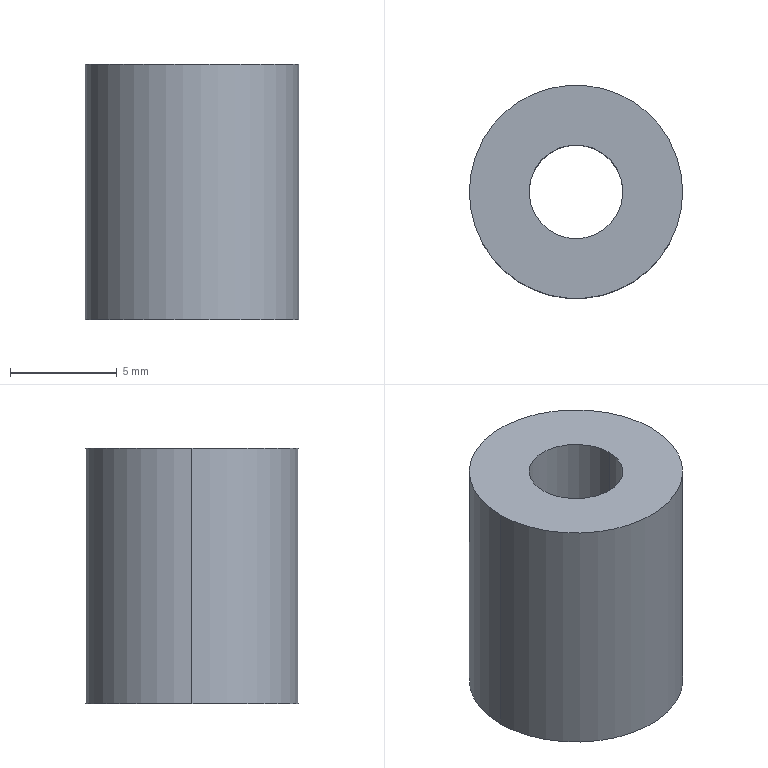Part | SolidWorks | features Extrusion 1 | 1 solid | 6 faces | box 10 x 10 x 12 mm | volume 760.014 mm3 | cylinder 4 | plane 2 | commonest cylinder face diameters 4.4 x2 10 x2
STEP:
#1=CARTESIAN_POINT('',(-2.2,0.,-6.));
#2=VERTEX_POINT('',#1);
#3=CARTESIAN_POINT('',(2.2,0.,-6.));
#4=VERTEX_POINT('',#3);
#5=CARTESIAN_POINT('',(0.,0.,-6.));
#6=DIRECTION('',(0.,0.,1.));
#7=DIRECTION('',(1.,0.,0.));
#8=AXIS2_PLACEMENT_3D('',#5,#6,#7);
#9=CIRCLE('',#8,2.2);
#10=EDGE_CURVE('',#2,#4,#9,.T.);
#11=ORIENTED_EDGE('',*,*,#10,.F.);
#12=CARTESIAN_POINT('',(-2.2,0.,6.));
#13=VERTEX_POINT('',#12);
#14=CARTESIAN_POINT('',(-2.2,0.,-6.));
#15=DIRECTION('',(0.,0.,1.));
#16=VECTOR('',#15,1000.);
#17=LINE('',#14,#16);
#18=EDGE_CURVE('',#2,#13,#17,.T.);
#19=ORIENTED_EDGE('',*,*,#18,.T.);
#20=CARTESIAN_POINT('',(2.2,0.,6.));
#21=VERTEX_POINT('',#20);
#22=CARTESIAN_POINT('',(0.,0.,6.));
#23=DIRECTION('',(0.,0.,1.));
#24=DIRECTION('',(1.,0.,0.));
#25=AXIS2_PLACEMENT_3D('',#22,#23,#24);
#26=CIRCLE('',#25,2.2);
#27=EDGE_CURVE('',#13,#21,#26,.T.);
#28=ORIENTED_EDGE('',*,*,#27,.T.);
#29=CARTESIAN_POINT('',(2.2,0.,-6.));
#30=DIRECTION('',(0.,0.,1.));
#31=VECTOR('',#30,1000.);
#32=LINE('',#29,#31);
#33=EDGE_CURVE('',#4,#21,#32,.T.);
#34=ORIENTED_EDGE('',*,*,#33,.F.);
#35=EDGE_LOOP('',(#11,#19,#28,#34));
#36=FACE_OUTER_BOUND('',#35,.T.);
#37=CARTESIAN_POINT('',(0.,0.,-6.));
#38=DIRECTION('',(0.,0.,1.));
#39=DIRECTION('',(1.,0.,0.));
#40=AXIS2_PLACEMENT_3D('',#37,#38,#39);
#41=CYLINDRICAL_SURFACE('',#40,2.2);
#42=ADVANCED_FACE('',(#36),#41,.F.);
#43=CARTESIAN_POINT('',(5.,0.,-6.));
#44=VERTEX_POINT('',#43);
#45=CARTESIAN_POINT('',(-5.,0.,-6.));
#46=VERTEX_POINT('',#45);
#47=CARTESIAN_POINT('',(0.,0.,-6.));
#48=DIRECTION('',(0.,0.,1.));
#49=DIRECTION('',(1.,0.,0.));
#50=AXIS2_PLACEMENT_3D('',#47,#48,#49);
#51=CIRCLE('',#50,5.);
#52=EDGE_CURVE('',#44,#46,#51,.T.);
#53=ORIENTED_EDGE('',*,*,#52,.T.);
#54=CARTESIAN_POINT('',(-5.,0.,6.));
#55=VERTEX_POINT('',#54);
#56=CARTESIAN_POINT('',(-5.,0.,-6.));
#57=DIRECTION('',(0.,0.,1.));
#58=VECTOR('',#57,1000.);
#59=LINE('',#56,#58);
#60=EDGE_CURVE('',#46,#55,#59,.T.);
#61=ORIENTED_EDGE('',*,*,#60,.T.);
#62=CARTESIAN_POINT('',(5.,0.,6.));
#63=VERTEX_POINT('',#62);
#64=CARTESIAN_POINT('',(0.,0.,6.));
#65=DIRECTION('',(0.,0.,1.));
#66=DIRECTION('',(1.,0.,0.));
#67=AXIS2_PLACEMENT_3D('',#64,#65,#66);
#68=CIRCLE('',#67,5.);
#69=EDGE_CURVE('',#63,#55,#68,.T.);
#70=ORIENTED_EDGE('',*,*,#69,.F.);
#71=CARTESIAN_POINT('',(5.,0.,-6.));
#72=DIRECTION('',(0.,0.,1.));
#73=VECTOR('',#72,1000.);
#74=LINE('',#71,#73);
#75=EDGE_CURVE('',#44,#63,#74,.T.);
#76=ORIENTED_EDGE('',*,*,#75,.F.);
#77=EDGE_LOOP('',(#53,#61,#70,#76));
#78=FACE_OUTER_BOUND('',#77,.T.);
#79=CARTESIAN_POINT('',(0.,0.,-6.));
#80=DIRECTION('',(0.,0.,1.));
#81=DIRECTION('',(1.,0.,0.));
#82=AXIS2_PLACEMENT_3D('',#79,#80,#81);
#83=CYLINDRICAL_SURFACE('',#82,5.);
#84=ADVANCED_FACE('',(#78),#83,.T.);
#85=ORIENTED_EDGE('',*,*,#60,.F.);
#86=CARTESIAN_POINT('',(0.,0.,-6.));
#87=DIRECTION('',(0.,0.,1.));
#88=DIRECTION('',(1.,0.,0.));
#89=AXIS2_PLACEMENT_3D('',#86,#87,#88);
#90=CIRCLE('',#89,5.);
#91=EDGE_CURVE('',#46,#44,#90,.T.);
#92=ORIENTED_EDGE('',*,*,#91,.T.);
#93=ORIENTED_EDGE('',*,*,#75,.T.);
#94=CARTESIAN_POINT('',(0.,0.,6.));
#95=DIRECTION('',(0.,0.,1.));
#96=DIRECTION('',(1.,0.,0.));
#97=AXIS2_PLACEMENT_3D('',#94,#95,#96);
#98=CIRCLE('',#97,5.);
#99=EDGE_CURVE('',#55,#63,#98,.T.);
#100=ORIENTED_EDGE('',*,*,#99,.F.);
#101=EDGE_LOOP('',(#85,#92,#93,#100));
#102=FACE_OUTER_BOUND('',#101,.T.);
#103=CARTESIAN_POINT('',(0.,0.,-6.));
#104=DIRECTION('',(0.,0.,1.));
#105=DIRECTION('',(1.,0.,0.));
#106=AXIS2_PLACEMENT_3D('',#103,#104,#105);
#107=CYLINDRICAL_SURFACE('',#106,5.);
#108=ADVANCED_FACE('',(#102),#107,.T.);
#109=CARTESIAN_POINT('',(0.,0.,-6.));
#110=DIRECTION('',(0.,0.,1.));
#111=DIRECTION('',(1.,0.,0.));
#112=AXIS2_PLACEMENT_3D('',#109,#110,#111);
#113=CIRCLE('',#112,2.2);
#114=EDGE_CURVE('',#4,#2,#113,.T.);
#115=ORIENTED_EDGE('',*,*,#114,.T.);
#116=ORIENTED_EDGE('',*,*,#10,.T.);
#117=EDGE_LOOP('',(#115,#116));
#118=FACE_BOUND('',#117,.T.);
#119=ORIENTED_EDGE('',*,*,#52,.F.);
#120=ORIENTED_EDGE('',*,*,#91,.F.);
#121=EDGE_LOOP('',(#119,#120));
#122=FACE_OUTER_BOUND('',#121,.T.);
#123=CARTESIAN_POINT('',(0.,0.,-6.));
#124=DIRECTION('',(0.,0.,1.));
#125=DIRECTION('',(1.,0.,0.));
#126=AXIS2_PLACEMENT_3D('',#123,#124,#125);
#127=PLANE('',#126);
#128=ADVANCED_FACE('',(#118,#122),#127,.F.);
#129=CARTESIAN_POINT('',(0.,0.,6.));
#130=DIRECTION('',(0.,0.,1.));
#131=DIRECTION('',(1.,0.,0.));
#132=AXIS2_PLACEMENT_3D('',#129,#130,#131);
#133=CIRCLE('',#132,2.2);
#134=EDGE_CURVE('',#21,#13,#133,.T.);
#135=ORIENTED_EDGE('',*,*,#134,.F.);
#136=ORIENTED_EDGE('',*,*,#27,.F.);
#137=EDGE_LOOP('',(#135,#136));
#138=FACE_BOUND('',#137,.T.);
#139=ORIENTED_EDGE('',*,*,#69,.T.);
#140=ORIENTED_EDGE('',*,*,#99,.T.);
#141=EDGE_LOOP('',(#139,#140));
#142=FACE_OUTER_BOUND('',#141,.T.);
#143=CARTESIAN_POINT('',(0.,0.,6.));
#144=DIRECTION('',(0.,0.,1.));
#145=DIRECTION('',(1.,0.,0.));
#146=AXIS2_PLACEMENT_3D('',#143,#144,#145);
#147=PLANE('',#146);
#148=ADVANCED_FACE('',(#138,#142),#147,.T.);
#149=ORIENTED_EDGE('',*,*,#18,.F.);
#150=ORIENTED_EDGE('',*,*,#114,.F.);
#151=ORIENTED_EDGE('',*,*,#33,.T.);
#152=ORIENTED_EDGE('',*,*,#134,.T.);
#153=EDGE_LOOP('',(#149,#150,#151,#152));
#154=FACE_OUTER_BOUND('',#153,.T.);
#155=CARTESIAN_POINT('',(0.,0.,-6.));
#156=DIRECTION('',(0.,0.,1.));
#157=DIRECTION('',(1.,0.,0.));
#158=AXIS2_PLACEMENT_3D('',#155,#156,#157);
#159=CYLINDRICAL_SURFACE('',#158,2.2);
#160=ADVANCED_FACE('',(#154),#159,.F.);
#161=CLOSED_SHELL('',(#42,#84,#108,#128,#148,#160));
#162=MANIFOLD_SOLID_BREP('',#161);
#163=CARTESIAN_POINT('',(0.,0.,0.));
#164=DIRECTION('',(0.,0.,1.));
#165=DIRECTION('',(1.,0.,0.));
#166=AXIS2_PLACEMENT_3D('',#163,#164,#165);
#167=(LENGTH_UNIT()NAMED_UNIT(*)SI_UNIT(.MILLI.,.METRE.));
#168=UNCERTAINTY_MEASURE_WITH_UNIT(LENGTH_MEASURE(0.00001),#167,'','');
#169=(NAMED_UNIT(*)PLANE_ANGLE_UNIT()SI_UNIT($,.RADIAN.));
#170=(NAMED_UNIT(*)SI_UNIT($,.STERADIAN.)SOLID_ANGLE_UNIT());
#171=(GEOMETRIC_REPRESENTATION_CONTEXT(3)GLOBAL_UNCERTAINTY_ASSIGNED_CONTEXT((#168))GLOBAL_UNIT_ASSIGNED_CONTEXT((#167,#169,#170))REPRESENTATION_CONTEXT('',''));
#172=ADVANCED_BREP_SHAPE_REPRESENTATION('',(#162,#166),#171);